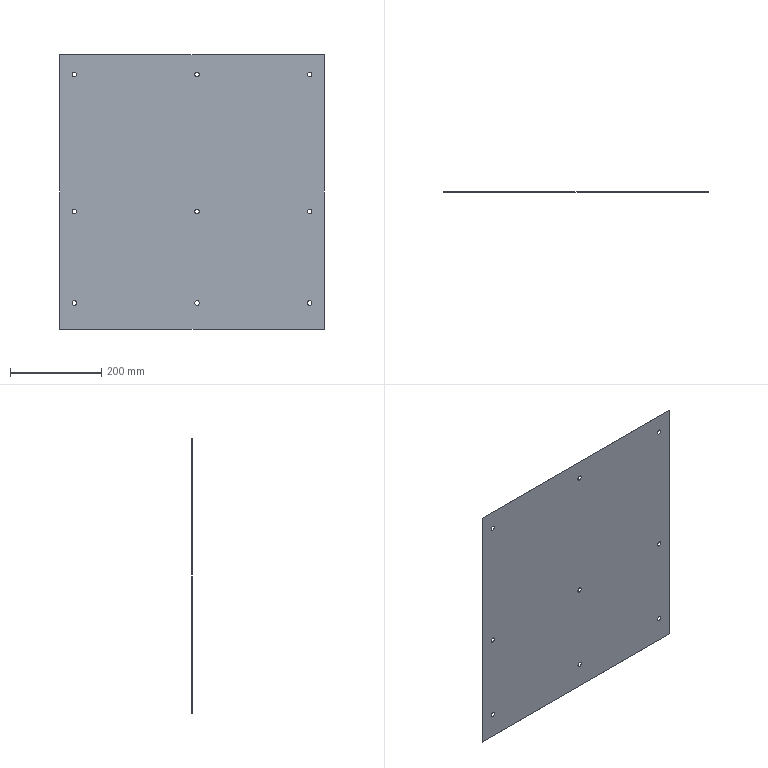Part | SolidWorks | features LPattern 2, Extrusion 1, FlatPattern 1, HoleWzd 1, SheetMetal 1, SolidToSheetMetal 1 | 1 solid | 24 faces | box 580 x 0.18 x 600 mm | volume 62513 mm3 | cylinder 18 | plane 6 | commonest cylinder face diameters 10 x18
STEP:
#1=CARTESIAN_POINT('',(301.2,0.18,52.));
#2=VERTEX_POINT('',#1);
#3=CARTESIAN_POINT('',(301.2,0.18,62.));
#4=VERTEX_POINT('',#3);
#5=CARTESIAN_POINT('',(301.2,0.18,57.));
#6=DIRECTION('',(0.,1.,0.));
#7=DIRECTION('',(0.,0.,1.));
#8=AXIS2_PLACEMENT_3D('',#5,#6,#7);
#9=CIRCLE('',#8,5.);
#10=EDGE_CURVE('',#2,#4,#9,.T.);
#11=ORIENTED_EDGE('',*,*,#10,.T.);
#12=CARTESIAN_POINT('',(301.2,0.,62.));
#13=VERTEX_POINT('',#12);
#14=CARTESIAN_POINT('',(301.2,0.,62.));
#15=DIRECTION('',(0.,-1.,0.));
#16=VECTOR('',#15,1000.);
#17=LINE('',#14,#16);
#18=EDGE_CURVE('',#4,#13,#17,.T.);
#19=ORIENTED_EDGE('',*,*,#18,.T.);
#20=CARTESIAN_POINT('',(301.2,0.,52.));
#21=VERTEX_POINT('',#20);
#22=CARTESIAN_POINT('',(301.2,0.,57.));
#23=DIRECTION('',(0.,-1.,0.));
#24=DIRECTION('',(0.,0.,-1.));
#25=AXIS2_PLACEMENT_3D('',#22,#23,#24);
#26=CIRCLE('',#25,5.);
#27=EDGE_CURVE('',#13,#21,#26,.T.);
#28=ORIENTED_EDGE('',*,*,#27,.T.);
#29=CARTESIAN_POINT('',(301.2,0.,52.));
#30=DIRECTION('',(0.,-1.,0.));
#31=VECTOR('',#30,1000.);
#32=LINE('',#29,#31);
#33=EDGE_CURVE('',#2,#21,#32,.T.);
#34=ORIENTED_EDGE('',*,*,#33,.F.);
#35=EDGE_LOOP('',(#11,#19,#28,#34));
#36=FACE_OUTER_BOUND('',#35,.T.);
#37=CARTESIAN_POINT('',(301.2,0.,57.));
#38=DIRECTION('',(0.,-1.,0.));
#39=DIRECTION('',(0.,0.,-1.));
#40=AXIS2_PLACEMENT_3D('',#37,#38,#39);
#41=CYLINDRICAL_SURFACE('',#40,5.);
#42=ADVANCED_FACE('',(#36),#41,.F.);
#43=CARTESIAN_POINT('',(32.4,0.18,52.));
#44=VERTEX_POINT('',#43);
#45=CARTESIAN_POINT('',(32.4,0.18,62.));
#46=VERTEX_POINT('',#45);
#47=CARTESIAN_POINT('',(32.4,0.18,57.));
#48=DIRECTION('',(0.,1.,0.));
#49=DIRECTION('',(0.,0.,1.));
#50=AXIS2_PLACEMENT_3D('',#47,#48,#49);
#51=CIRCLE('',#50,5.);
#52=EDGE_CURVE('',#44,#46,#51,.T.);
#53=ORIENTED_EDGE('',*,*,#52,.T.);
#54=CARTESIAN_POINT('',(32.4,0.,62.));
#55=VERTEX_POINT('',#54);
#56=CARTESIAN_POINT('',(32.4,0.,62.));
#57=DIRECTION('',(0.,-1.,0.));
#58=VECTOR('',#57,1000.);
#59=LINE('',#56,#58);
#60=EDGE_CURVE('',#46,#55,#59,.T.);
#61=ORIENTED_EDGE('',*,*,#60,.T.);
#62=CARTESIAN_POINT('',(32.4,0.,52.));
#63=VERTEX_POINT('',#62);
#64=CARTESIAN_POINT('',(32.4,0.,57.));
#65=DIRECTION('',(0.,-1.,0.));
#66=DIRECTION('',(0.,0.,-1.));
#67=AXIS2_PLACEMENT_3D('',#64,#65,#66);
#68=CIRCLE('',#67,5.);
#69=EDGE_CURVE('',#55,#63,#68,.T.);
#70=ORIENTED_EDGE('',*,*,#69,.T.);
#71=CARTESIAN_POINT('',(32.4,0.,52.));
#72=DIRECTION('',(0.,-1.,0.));
#73=VECTOR('',#72,1000.);
#74=LINE('',#71,#73);
#75=EDGE_CURVE('',#44,#63,#74,.T.);
#76=ORIENTED_EDGE('',*,*,#75,.F.);
#77=EDGE_LOOP('',(#53,#61,#70,#76));
#78=FACE_OUTER_BOUND('',#77,.T.);
#79=CARTESIAN_POINT('',(32.4,0.,57.));
#80=DIRECTION('',(0.,-1.,0.));
#81=DIRECTION('',(0.,0.,-1.));
#82=AXIS2_PLACEMENT_3D('',#79,#80,#81);
#83=CYLINDRICAL_SURFACE('',#82,5.);
#84=ADVANCED_FACE('',(#78),#83,.F.);
#85=CARTESIAN_POINT('',(547.6,0.18,52.));
#86=VERTEX_POINT('',#85);
#87=CARTESIAN_POINT('',(547.6,0.18,62.));
#88=VERTEX_POINT('',#87);
#89=CARTESIAN_POINT('',(547.6,0.18,57.));
#90=DIRECTION('',(0.,1.,0.));
#91=DIRECTION('',(0.,0.,1.));
#92=AXIS2_PLACEMENT_3D('',#89,#90,#91);
#93=CIRCLE('',#92,5.);
#94=EDGE_CURVE('',#86,#88,#93,.T.);
#95=ORIENTED_EDGE('',*,*,#94,.T.);
#96=CARTESIAN_POINT('',(547.6,0.,62.));
#97=VERTEX_POINT('',#96);
#98=CARTESIAN_POINT('',(547.6,0.,62.));
#99=DIRECTION('',(0.,-1.,0.));
#100=VECTOR('',#99,1000.);
#101=LINE('',#98,#100);
#102=EDGE_CURVE('',#88,#97,#101,.T.);
#103=ORIENTED_EDGE('',*,*,#102,.T.);
#104=CARTESIAN_POINT('',(547.6,0.,52.));
#105=VERTEX_POINT('',#104);
#106=CARTESIAN_POINT('',(547.6,0.,57.));
#107=DIRECTION('',(0.,-1.,0.));
#108=DIRECTION('',(0.,0.,-1.));
#109=AXIS2_PLACEMENT_3D('',#106,#107,#108);
#110=CIRCLE('',#109,5.);
#111=EDGE_CURVE('',#97,#105,#110,.T.);
#112=ORIENTED_EDGE('',*,*,#111,.T.);
#113=CARTESIAN_POINT('',(547.6,0.,52.));
#114=DIRECTION('',(0.,-1.,0.));
#115=VECTOR('',#114,1000.);
#116=LINE('',#113,#115);
#117=EDGE_CURVE('',#86,#105,#116,.T.);
#118=ORIENTED_EDGE('',*,*,#117,.F.);
#119=EDGE_LOOP('',(#95,#103,#112,#118));
#120=FACE_OUTER_BOUND('',#119,.T.);
#121=CARTESIAN_POINT('',(547.6,0.,57.));
#122=DIRECTION('',(0.,-1.,0.));
#123=DIRECTION('',(0.,0.,-1.));
#124=AXIS2_PLACEMENT_3D('',#121,#122,#123);
#125=CYLINDRICAL_SURFACE('',#124,5.);
#126=ADVANCED_FACE('',(#120),#125,.F.);
#127=CARTESIAN_POINT('',(301.2,0.18,252.));
#128=VERTEX_POINT('',#127);
#129=CARTESIAN_POINT('',(301.2,0.18,262.));
#130=VERTEX_POINT('',#129);
#131=CARTESIAN_POINT('',(301.2,0.18,257.));
#132=DIRECTION('',(0.,1.,0.));
#133=DIRECTION('',(0.,0.,1.));
#134=AXIS2_PLACEMENT_3D('',#131,#132,#133);
#135=CIRCLE('',#134,5.);
#136=EDGE_CURVE('',#128,#130,#135,.T.);
#137=ORIENTED_EDGE('',*,*,#136,.T.);
#138=CARTESIAN_POINT('',(301.2,0.,262.));
#139=VERTEX_POINT('',#138);
#140=CARTESIAN_POINT('',(301.2,0.,262.));
#141=DIRECTION('',(0.,-1.,0.));
#142=VECTOR('',#141,1000.);
#143=LINE('',#140,#142);
#144=EDGE_CURVE('',#130,#139,#143,.T.);
#145=ORIENTED_EDGE('',*,*,#144,.T.);
#146=CARTESIAN_POINT('',(301.2,0.,252.));
#147=VERTEX_POINT('',#146);
#148=CARTESIAN_POINT('',(301.2,0.,257.));
#149=DIRECTION('',(0.,-1.,0.));
#150=DIRECTION('',(0.,0.,-1.));
#151=AXIS2_PLACEMENT_3D('',#148,#149,#150);
#152=CIRCLE('',#151,5.);
#153=EDGE_CURVE('',#139,#147,#152,.T.);
#154=ORIENTED_EDGE('',*,*,#153,.T.);
#155=CARTESIAN_POINT('',(301.2,0.,252.));
#156=DIRECTION('',(0.,-1.,0.));
#157=VECTOR('',#156,1000.);
#158=LINE('',#155,#157);
#159=EDGE_CURVE('',#128,#147,#158,.T.);
#160=ORIENTED_EDGE('',*,*,#159,.F.);
#161=EDGE_LOOP('',(#137,#145,#154,#160));
#162=FACE_OUTER_BOUND('',#161,.T.);
#163=CARTESIAN_POINT('',(301.2,0.,257.));
#164=DIRECTION('',(0.,-1.,0.));
#165=DIRECTION('',(0.,0.,-1.));
#166=AXIS2_PLACEMENT_3D('',#163,#164,#165);
#167=CYLINDRICAL_SURFACE('',#166,5.);
#168=ADVANCED_FACE('',(#162),#167,.F.);
#169=CARTESIAN_POINT('',(32.4,0.18,252.));
#170=VERTEX_POINT('',#169);
#171=CARTESIAN_POINT('',(32.4,0.18,262.));
#172=VERTEX_POINT('',#171);
#173=CARTESIAN_POINT('',(32.4,0.18,257.));
#174=DIRECTION('',(0.,1.,0.));
#175=DIRECTION('',(0.,0.,1.));
#176=AXIS2_PLACEMENT_3D('',#173,#174,#175);
#177=CIRCLE('',#176,5.);
#178=EDGE_CURVE('',#170,#172,#177,.T.);
#179=ORIENTED_EDGE('',*,*,#178,.T.);
#180=CARTESIAN_POINT('',(32.4,0.,262.));
#181=VERTEX_POINT('',#180);
#182=CARTESIAN_POINT('',(32.4,0.,262.));
#183=DIRECTION('',(0.,-1.,0.));
#184=VECTOR('',#183,1000.);
#185=LINE('',#182,#184);
#186=EDGE_CURVE('',#172,#181,#185,.T.);
#187=ORIENTED_EDGE('',*,*,#186,.T.);
#188=CARTESIAN_POINT('',(32.4,0.,252.));
#189=VERTEX_POINT('',#188);
#190=CARTESIAN_POINT('',(32.4,0.,257.));
#191=DIRECTION('',(0.,-1.,0.));
#192=DIRECTION('',(0.,0.,-1.));
#193=AXIS2_PLACEMENT_3D('',#190,#191,#192);
#194=CIRCLE('',#193,5.);
#195=EDGE_CURVE('',#181,#189,#194,.T.);
#196=ORIENTED_EDGE('',*,*,#195,.T.);
#197=CARTESIAN_POINT('',(32.4,0.,252.));
#198=DIRECTION('',(0.,-1.,0.));
#199=VECTOR('',#198,1000.);
#200=LINE('',#197,#199);
#201=EDGE_CURVE('',#170,#189,#200,.T.);
#202=ORIENTED_EDGE('',*,*,#201,.F.);
#203=EDGE_LOOP('',(#179,#187,#196,#202));
#204=FACE_OUTER_BOUND('',#203,.T.);
#205=CARTESIAN_POINT('',(32.4,0.,257.));
#206=DIRECTION('',(0.,-1.,0.));
#207=DIRECTION('',(0.,0.,-1.));
#208=AXIS2_PLACEMENT_3D('',#205,#206,#207);
#209=CYLINDRICAL_SURFACE('',#208,5.);
#210=ADVANCED_FACE('',(#204),#209,.F.);
#211=CARTESIAN_POINT('',(547.6,0.18,252.));
#212=VERTEX_POINT('',#211);
#213=CARTESIAN_POINT('',(547.6,0.18,262.));
#214=VERTEX_POINT('',#213);
#215=CARTESIAN_POINT('',(547.6,0.18,257.));
#216=DIRECTION('',(0.,1.,0.));
#217=DIRECTION('',(0.,0.,1.));
#218=AXIS2_PLACEMENT_3D('',#215,#216,#217);
#219=CIRCLE('',#218,5.);
#220=EDGE_CURVE('',#212,#214,#219,.T.);
#221=ORIENTED_EDGE('',*,*,#220,.T.);
#222=CARTESIAN_POINT('',(547.6,0.,262.));
#223=VERTEX_POINT('',#222);
#224=CARTESIAN_POINT('',(547.6,0.,262.));
#225=DIRECTION('',(0.,-1.,0.));
#226=VECTOR('',#225,1000.);
#227=LINE('',#224,#226);
#228=EDGE_CURVE('',#214,#223,#227,.T.);
#229=ORIENTED_EDGE('',*,*,#228,.T.);
#230=CARTESIAN_POINT('',(547.6,0.,252.));
#231=VERTEX_POINT('',#230);
#232=CARTESIAN_POINT('',(547.6,0.,257.));
#233=DIRECTION('',(0.,-1.,0.));
#234=DIRECTION('',(0.,0.,-1.));
#235=AXIS2_PLACEMENT_3D('',#232,#233,#234);
#236=CIRCLE('',#235,5.);
#237=EDGE_CURVE('',#223,#231,#236,.T.);
#238=ORIENTED_EDGE('',*,*,#237,.T.);
#239=CARTESIAN_POINT('',(547.6,0.,252.));
#240=DIRECTION('',(0.,-1.,0.));
#241=VECTOR('',#240,1000.);
#242=LINE('',#239,#241);
#243=EDGE_CURVE('',#212,#231,#242,.T.);
#244=ORIENTED_EDGE('',*,*,#243,.F.);
#245=EDGE_LOOP('',(#221,#229,#238,#244));
#246=FACE_OUTER_BOUND('',#245,.T.);
#247=CARTESIAN_POINT('',(547.6,0.,257.));
#248=DIRECTION('',(0.,-1.,0.));
#249=DIRECTION('',(0.,0.,-1.));
#250=AXIS2_PLACEMENT_3D('',#247,#248,#249);
#251=CYLINDRICAL_SURFACE('',#250,5.);
#252=ADVANCED_FACE('',(#246),#251,.F.);
#253=CARTESIAN_POINT('',(547.6,0.18,552.));
#254=VERTEX_POINT('',#253);
#255=CARTESIAN_POINT('',(547.6,0.18,562.));
#256=VERTEX_POINT('',#255);
#257=CARTESIAN_POINT('',(547.6,0.18,557.));
#258=DIRECTION('',(0.,1.,0.));
#259=DIRECTION('',(0.,0.,1.));
#260=AXIS2_PLACEMENT_3D('',#257,#258,#259);
#261=CIRCLE('',#260,5.);
#262=EDGE_CURVE('',#254,#256,#261,.T.);
#263=ORIENTED_EDGE('',*,*,#262,.T.);
#264=CARTESIAN_POINT('',(547.6,0.,562.));
#265=VERTEX_POINT('',#264);
#266=CARTESIAN_POINT('',(547.6,0.,562.));
#267=DIRECTION('',(0.,-1.,0.));
#268=VECTOR('',#267,1000.);
#269=LINE('',#266,#268);
#270=EDGE_CURVE('',#256,#265,#269,.T.);
#271=ORIENTED_EDGE('',*,*,#270,.T.);
#272=CARTESIAN_POINT('',(547.6,0.,552.));
#273=VERTEX_POINT('',#272);
#274=CARTESIAN_POINT('',(547.6,0.,557.));
#275=DIRECTION('',(0.,-1.,0.));
#276=DIRECTION('',(0.,0.,-1.));
#277=AXIS2_PLACEMENT_3D('',#274,#275,#276);
#278=CIRCLE('',#277,5.);
#279=EDGE_CURVE('',#265,#273,#278,.T.);
#280=ORIENTED_EDGE('',*,*,#279,.T.);
#281=CARTESIAN_POINT('',(547.6,0.,552.));
#282=DIRECTION('',(0.,-1.,0.));
#283=VECTOR('',#282,1000.);
#284=LINE('',#281,#283);
#285=EDGE_CURVE('',#254,#273,#284,.T.);
#286=ORIENTED_EDGE('',*,*,#285,.F.);
#287=EDGE_LOOP('',(#263,#271,#280,#286));
#288=FACE_OUTER_BOUND('',#287,.T.);
#289=CARTESIAN_POINT('',(547.6,0.,557.));
#290=DIRECTION('',(0.,-1.,0.));
#291=DIRECTION('',(0.,0.,-1.));
#292=AXIS2_PLACEMENT_3D('',#289,#290,#291);
#293=CYLINDRICAL_SURFACE('',#292,5.);
#294=ADVANCED_FACE('',(#288),#293,.F.);
#295=CARTESIAN_POINT('',(301.2,0.18,552.));
#296=VERTEX_POINT('',#295);
#297=CARTESIAN_POINT('',(301.2,0.18,562.));
#298=VERTEX_POINT('',#297);
#299=CARTESIAN_POINT('',(301.2,0.18,557.));
#300=DIRECTION('',(0.,1.,0.));
#301=DIRECTION('',(0.,0.,1.));
#302=AXIS2_PLACEMENT_3D('',#299,#300,#301);
#303=CIRCLE('',#302,5.);
#304=EDGE_CURVE('',#296,#298,#303,.T.);
#305=ORIENTED_EDGE('',*,*,#304,.T.);
#306=CARTESIAN_POINT('',(301.2,0.,562.));
#307=VERTEX_POINT('',#306);
#308=CARTESIAN_POINT('',(301.2,0.,562.));
#309=DIRECTION('',(0.,-1.,0.));
#310=VECTOR('',#309,1000.);
#311=LINE('',#308,#310);
#312=EDGE_CURVE('',#298,#307,#311,.T.);
#313=ORIENTED_EDGE('',*,*,#312,.T.);
#314=CARTESIAN_POINT('',(301.2,0.,552.));
#315=VERTEX_POINT('',#314);
#316=CARTESIAN_POINT('',(301.2,0.,557.));
#317=DIRECTION('',(0.,-1.,0.));
#318=DIRECTION('',(0.,0.,-1.));
#319=AXIS2_PLACEMENT_3D('',#316,#317,#318);
#320=CIRCLE('',#319,5.);
#321=EDGE_CURVE('',#307,#315,#320,.T.);
#322=ORIENTED_EDGE('',*,*,#321,.T.);
#323=CARTESIAN_POINT('',(301.2,0.,552.));
#324=DIRECTION('',(0.,-1.,0.));
#325=VECTOR('',#324,1000.);
#326=LINE('',#323,#325);
#327=EDGE_CURVE('',#296,#315,#326,.T.);
#328=ORIENTED_EDGE('',*,*,#327,.F.);
#329=EDGE_LOOP('',(#305,#313,#322,#328));
#330=FACE_OUTER_BOUND('',#329,.T.);
#331=CARTESIAN_POINT('',(301.2,0.,557.));
#332=DIRECTION('',(0.,-1.,0.));
#333=DIRECTION('',(0.,0.,-1.));
#334=AXIS2_PLACEMENT_3D('',#331,#332,#333);
#335=CYLINDRICAL_SURFACE('',#334,5.);
#336=ADVANCED_FACE('',(#330),#335,.F.);
#337=CARTESIAN_POINT('',(32.4,0.18,552.));
#338=VERTEX_POINT('',#337);
#339=CARTESIAN_POINT('',(32.4,0.18,562.));
#340=VERTEX_POINT('',#339);
#341=CARTESIAN_POINT('',(32.4,0.18,557.));
#342=DIRECTION('',(0.,1.,0.));
#343=DIRECTION('',(0.,0.,1.));
#344=AXIS2_PLACEMENT_3D('',#341,#342,#343);
#345=CIRCLE('',#344,5.);
#346=EDGE_CURVE('',#338,#340,#345,.T.);
#347=ORIENTED_EDGE('',*,*,#346,.T.);
#348=CARTESIAN_POINT('',(32.4,0.,562.));
#349=VERTEX_POINT('',#348);
#350=CARTESIAN_POINT('',(32.4,0.,562.));
#351=DIRECTION('',(0.,-1.,0.));
#352=VECTOR('',#351,1000.);
#353=LINE('',#350,#352);
#354=EDGE_CURVE('',#340,#349,#353,.T.);
#355=ORIENTED_EDGE('',*,*,#354,.T.);
#356=CARTESIAN_POINT('',(32.4,0.,552.));
#357=VERTEX_POINT('',#356);
#358=CARTESIAN_POINT('',(32.4,0.,557.));
#359=DIRECTION('',(0.,-1.,0.));
#360=DIRECTION('',(0.,0.,-1.));
#361=AXIS2_PLACEMENT_3D('',#358,#359,#360);
#362=CIRCLE('',#361,5.);
#363=EDGE_CURVE('',#349,#357,#362,.T.);
#364=ORIENTED_EDGE('',*,*,#363,.T.);
#365=CARTESIAN_POINT('',(32.4,0.,552.));
#366=DIRECTION('',(0.,-1.,0.));
#367=VECTOR('',#366,1000.);
#368=LINE('',#365,#367);
#369=EDGE_CURVE('',#338,#357,#368,.T.);
#370=ORIENTED_EDGE('',*,*,#369,.F.);
#371=EDGE_LOOP('',(#347,#355,#364,#370));
#372=FACE_OUTER_BOUND('',#371,.T.);
#373=CARTESIAN_POINT('',(32.4,0.,557.));
#374=DIRECTION('',(0.,-1.,0.));
#375=DIRECTION('',(0.,0.,-1.));
#376=AXIS2_PLACEMENT_3D('',#373,#374,#375);
#377=CYLINDRICAL_SURFACE('',#376,5.);
#378=ADVANCED_FACE('',(#372),#377,.F.);
#379=CARTESIAN_POINT('',(580.,0.,600.));
#380=VERTEX_POINT('',#379);
#381=CARTESIAN_POINT('',(580.,0.18,600.));
#382=VERTEX_POINT('',#381);
#383=CARTESIAN_POINT('',(580.,0.18,600.));
#384=DIRECTION('',(0.,1.,0.));
#385=VECTOR('',#384,1000.);
#386=LINE('',#383,#385);
#387=EDGE_CURVE('',#380,#382,#386,.T.);
#388=ORIENTED_EDGE('',*,*,#387,.F.);
#389=CARTESIAN_POINT('',(580.,0.,0.));
#390=VERTEX_POINT('',#389);
#391=CARTESIAN_POINT('',(580.,0.,0.));
#392=DIRECTION('',(0.,0.,-1.));
#393=VECTOR('',#392,1000.);
#394=LINE('',#391,#393);
#395=EDGE_CURVE('',#380,#390,#394,.T.);
#396=ORIENTED_EDGE('',*,*,#395,.T.);
#397=CARTESIAN_POINT('',(580.,0.18,0.));
#398=VERTEX_POINT('',#397);
#399=CARTESIAN_POINT('',(580.,0.18,0.));
#400=DIRECTION('',(0.,1.,0.));
#401=VECTOR('',#400,1000.);
#402=LINE('',#399,#401);
#403=EDGE_CURVE('',#390,#398,#402,.T.);
#404=ORIENTED_EDGE('',*,*,#403,.T.);
#405=CARTESIAN_POINT('',(580.,0.18,0.));
#406=DIRECTION('',(0.,0.,-1.));
#407=VECTOR('',#406,1000.);
#408=LINE('',#405,#407);
#409=EDGE_CURVE('',#382,#398,#408,.T.);
#410=ORIENTED_EDGE('',*,*,#409,.F.);
#411=EDGE_LOOP('',(#388,#396,#404,#410));
#412=FACE_OUTER_BOUND('',#411,.T.);
#413=CARTESIAN_POINT('',(580.,0.18,0.));
#414=DIRECTION('',(1.,0.,0.));
#415=DIRECTION('',(0.,0.,-1.));
#416=AXIS2_PLACEMENT_3D('',#413,#414,#415);
#417=PLANE('',#416);
#418=ADVANCED_FACE('',(#412),#417,.T.);
#419=ORIENTED_EDGE('',*,*,#403,.F.);
#420=CARTESIAN_POINT('',(0.,0.,0.));
#421=VERTEX_POINT('',#420);
#422=CARTESIAN_POINT('',(0.,0.,0.));
#423=DIRECTION('',(-1.,0.,0.));
#424=VECTOR('',#423,1000.);
#425=LINE('',#422,#424);
#426=EDGE_CURVE('',#390,#421,#425,.T.);
#427=ORIENTED_EDGE('',*,*,#426,.T.);
#428=CARTESIAN_POINT('',(0.,0.18,0.));
#429=VERTEX_POINT('',#428);
#430=CARTESIAN_POINT('',(0.,0.18,0.));
#431=DIRECTION('',(0.,1.,0.));
#432=VECTOR('',#431,1000.);
#433=LINE('',#430,#432);
#434=EDGE_CURVE('',#421,#429,#433,.T.);
#435=ORIENTED_EDGE('',*,*,#434,.T.);
#436=CARTESIAN_POINT('',(0.,0.18,0.));
#437=DIRECTION('',(-1.,0.,0.));
#438=VECTOR('',#437,1000.);
#439=LINE('',#436,#438);
#440=EDGE_CURVE('',#398,#429,#439,.T.);
#441=ORIENTED_EDGE('',*,*,#440,.F.);
#442=EDGE_LOOP('',(#419,#427,#435,#441));
#443=FACE_OUTER_BOUND('',#442,.T.);
#444=CARTESIAN_POINT('',(0.,0.18,0.));
#445=DIRECTION('',(0.,0.,-1.));
#446=DIRECTION('',(-1.,0.,0.));
#447=AXIS2_PLACEMENT_3D('',#444,#445,#446);
#448=PLANE('',#447);
#449=ADVANCED_FACE('',(#443),#448,.T.);
#450=ORIENTED_EDGE('',*,*,#434,.F.);
#451=CARTESIAN_POINT('',(0.,0.,600.));
#452=VERTEX_POINT('',#451);
#453=CARTESIAN_POINT('',(0.,0.,0.));
#454=DIRECTION('',(0.,0.,1.));
#455=VECTOR('',#454,1000.);
#456=LINE('',#453,#455);
#457=EDGE_CURVE('',#421,#452,#456,.T.);
#458=ORIENTED_EDGE('',*,*,#457,.T.);
#459=CARTESIAN_POINT('',(0.,0.18,600.));
#460=VERTEX_POINT('',#459);
#461=CARTESIAN_POINT('',(0.,0.18,600.));
#462=DIRECTION('',(0.,1.,0.));
#463=VECTOR('',#462,1000.);
#464=LINE('',#461,#463);
#465=EDGE_CURVE('',#452,#460,#464,.T.);
#466=ORIENTED_EDGE('',*,*,#465,.T.);
#467=CARTESIAN_POINT('',(0.,0.18,0.));
#468=DIRECTION('',(0.,0.,1.));
#469=VECTOR('',#468,1000.);
#470=LINE('',#467,#469);
#471=EDGE_CURVE('',#429,#460,#470,.T.);
#472=ORIENTED_EDGE('',*,*,#471,.F.);
#473=EDGE_LOOP('',(#450,#458,#466,#472));
#474=FACE_OUTER_BOUND('',#473,.T.);
#475=CARTESIAN_POINT('',(0.,0.18,0.));
#476=DIRECTION('',(-1.,0.,0.));
#477=DIRECTION('',(0.,0.,1.));
#478=AXIS2_PLACEMENT_3D('',#475,#476,#477);
#479=PLANE('',#478);
#480=ADVANCED_FACE('',(#474),#479,.T.);
#481=CARTESIAN_POINT('',(0.,0.,600.));
#482=DIRECTION('',(1.,0.,0.));
#483=VECTOR('',#482,1000.);
#484=LINE('',#481,#483);
#485=EDGE_CURVE('',#452,#380,#484,.T.);
#486=ORIENTED_EDGE('',*,*,#485,.T.);
#487=ORIENTED_EDGE('',*,*,#387,.T.);
#488=CARTESIAN_POINT('',(0.,0.18,600.));
#489=DIRECTION('',(1.,0.,0.));
#490=VECTOR('',#489,1000.);
#491=LINE('',#488,#490);
#492=EDGE_CURVE('',#460,#382,#491,.T.);
#493=ORIENTED_EDGE('',*,*,#492,.F.);
#494=ORIENTED_EDGE('',*,*,#465,.F.);
#495=EDGE_LOOP('',(#486,#487,#493,#494));
#496=FACE_OUTER_BOUND('',#495,.T.);
#497=CARTESIAN_POINT('',(0.,0.18,600.));
#498=DIRECTION('',(0.,0.,1.));
#499=DIRECTION('',(1.,0.,0.));
#500=AXIS2_PLACEMENT_3D('',#497,#498,#499);
#501=PLANE('',#500);
#502=ADVANCED_FACE('',(#496),#501,.T.);
#503=ORIENTED_EDGE('',*,*,#10,.F.);
#504=CARTESIAN_POINT('',(301.2,0.18,57.));
#505=DIRECTION('',(0.,1.,0.));
#506=DIRECTION('',(0.,0.,1.));
#507=AXIS2_PLACEMENT_3D('',#504,#505,#506);
#508=CIRCLE('',#507,5.);
#509=EDGE_CURVE('',#4,#2,#508,.T.);
#510=ORIENTED_EDGE('',*,*,#509,.F.);
#511=EDGE_LOOP('',(#503,#510));
#512=FACE_BOUND('',#511,.T.);
#513=ORIENTED_EDGE('',*,*,#52,.F.);
#514=CARTESIAN_POINT('',(32.4,0.18,57.));
#515=DIRECTION('',(0.,1.,0.));
#516=DIRECTION('',(0.,0.,1.));
#517=AXIS2_PLACEMENT_3D('',#514,#515,#516);
#518=CIRCLE('',#517,5.);
#519=EDGE_CURVE('',#46,#44,#518,.T.);
#520=ORIENTED_EDGE('',*,*,#519,.F.);
#521=EDGE_LOOP('',(#513,#520));
#522=FACE_BOUND('',#521,.T.);
#523=ORIENTED_EDGE('',*,*,#94,.F.);
#524=CARTESIAN_POINT('',(547.6,0.18,57.));
#525=DIRECTION('',(0.,1.,0.));
#526=DIRECTION('',(0.,0.,1.));
#527=AXIS2_PLACEMENT_3D('',#524,#525,#526);
#528=CIRCLE('',#527,5.);
#529=EDGE_CURVE('',#88,#86,#528,.T.);
#530=ORIENTED_EDGE('',*,*,#529,.F.);
#531=EDGE_LOOP('',(#523,#530));
#532=FACE_BOUND('',#531,.T.);
#533=ORIENTED_EDGE('',*,*,#136,.F.);
#534=CARTESIAN_POINT('',(301.2,0.18,257.));
#535=DIRECTION('',(0.,1.,0.));
#536=DIRECTION('',(0.,0.,1.));
#537=AXIS2_PLACEMENT_3D('',#534,#535,#536);
#538=CIRCLE('',#537,5.);
#539=EDGE_CURVE('',#130,#128,#538,.T.);
#540=ORIENTED_EDGE('',*,*,#539,.F.);
#541=EDGE_LOOP('',(#533,#540));
#542=FACE_BOUND('',#541,.T.);
#543=ORIENTED_EDGE('',*,*,#178,.F.);
#544=CARTESIAN_POINT('',(32.4,0.18,257.));
#545=DIRECTION('',(0.,1.,0.));
#546=DIRECTION('',(0.,0.,1.));
#547=AXIS2_PLACEMENT_3D('',#544,#545,#546);
#548=CIRCLE('',#547,5.);
#549=EDGE_CURVE('',#172,#170,#548,.T.);
#550=ORIENTED_EDGE('',*,*,#549,.F.);
#551=EDGE_LOOP('',(#543,#550));
#552=FACE_BOUND('',#551,.T.);
#553=ORIENTED_EDGE('',*,*,#220,.F.);
#554=CARTESIAN_POINT('',(547.6,0.18,257.));
#555=DIRECTION('',(0.,1.,0.));
#556=DIRECTION('',(0.,0.,1.));
#557=AXIS2_PLACEMENT_3D('',#554,#555,#556);
#558=CIRCLE('',#557,5.);
#559=EDGE_CURVE('',#214,#212,#558,.T.);
#560=ORIENTED_EDGE('',*,*,#559,.F.);
#561=EDGE_LOOP('',(#553,#560));
#562=FACE_BOUND('',#561,.T.);
#563=ORIENTED_EDGE('',*,*,#262,.F.);
#564=CARTESIAN_POINT('',(547.6,0.18,557.));
#565=DIRECTION('',(0.,1.,0.));
#566=DIRECTION('',(0.,0.,1.));
#567=AXIS2_PLACEMENT_3D('',#564,#565,#566);
#568=CIRCLE('',#567,5.);
#569=EDGE_CURVE('',#256,#254,#568,.T.);
#570=ORIENTED_EDGE('',*,*,#569,.F.);
#571=EDGE_LOOP('',(#563,#570));
#572=FACE_BOUND('',#571,.T.);
#573=ORIENTED_EDGE('',*,*,#304,.F.);
#574=CARTESIAN_POINT('',(301.2,0.18,557.));
#575=DIRECTION('',(0.,1.,0.));
#576=DIRECTION('',(0.,0.,1.));
#577=AXIS2_PLACEMENT_3D('',#574,#575,#576);
#578=CIRCLE('',#577,5.);
#579=EDGE_CURVE('',#298,#296,#578,.T.);
#580=ORIENTED_EDGE('',*,*,#579,.F.);
#581=EDGE_LOOP('',(#573,#580));
#582=FACE_BOUND('',#581,.T.);
#583=ORIENTED_EDGE('',*,*,#346,.F.);
#584=CARTESIAN_POINT('',(32.4,0.18,557.));
#585=DIRECTION('',(0.,1.,0.));
#586=DIRECTION('',(0.,0.,1.));
#587=AXIS2_PLACEMENT_3D('',#584,#585,#586);
#588=CIRCLE('',#587,5.);
#589=EDGE_CURVE('',#340,#338,#588,.T.);
#590=ORIENTED_EDGE('',*,*,#589,.F.);
#591=EDGE_LOOP('',(#583,#590));
#592=FACE_BOUND('',#591,.T.);
#593=ORIENTED_EDGE('',*,*,#471,.T.);
#594=ORIENTED_EDGE('',*,*,#492,.T.);
#595=ORIENTED_EDGE('',*,*,#409,.T.);
#596=ORIENTED_EDGE('',*,*,#440,.T.);
#597=EDGE_LOOP('',(#593,#594,#595,#596));
#598=FACE_OUTER_BOUND('',#597,.T.);
#599=CARTESIAN_POINT('',(0.,0.18,0.));
#600=DIRECTION('',(0.,1.,0.));
#601=DIRECTION('',(0.,0.,1.));
#602=AXIS2_PLACEMENT_3D('',#599,#600,#601);
#603=PLANE('',#602);
#604=ADVANCED_FACE('',(#512,#522,#532,#542,#552,#562,#572,#582,#592,#598),#603,.T.);
#605=CARTESIAN_POINT('',(301.2,0.,57.));
#606=DIRECTION('',(0.,-1.,0.));
#607=DIRECTION('',(0.,0.,-1.));
#608=AXIS2_PLACEMENT_3D('',#605,#606,#607);
#609=CIRCLE('',#608,5.);
#610=EDGE_CURVE('',#21,#13,#609,.T.);
#611=ORIENTED_EDGE('',*,*,#610,.F.);
#612=ORIENTED_EDGE('',*,*,#27,.F.);
#613=EDGE_LOOP('',(#611,#612));
#614=FACE_BOUND('',#613,.T.);
#615=CARTESIAN_POINT('',(32.4,0.,57.));
#616=DIRECTION('',(0.,-1.,0.));
#617=DIRECTION('',(0.,0.,-1.));
#618=AXIS2_PLACEMENT_3D('',#615,#616,#617);
#619=CIRCLE('',#618,5.);
#620=EDGE_CURVE('',#63,#55,#619,.T.);
#621=ORIENTED_EDGE('',*,*,#620,.F.);
#622=ORIENTED_EDGE('',*,*,#69,.F.);
#623=EDGE_LOOP('',(#621,#622));
#624=FACE_BOUND('',#623,.T.);
#625=CARTESIAN_POINT('',(547.6,0.,57.));
#626=DIRECTION('',(0.,-1.,0.));
#627=DIRECTION('',(0.,0.,-1.));
#628=AXIS2_PLACEMENT_3D('',#625,#626,#627);
#629=CIRCLE('',#628,5.);
#630=EDGE_CURVE('',#105,#97,#629,.T.);
#631=ORIENTED_EDGE('',*,*,#630,.F.);
#632=ORIENTED_EDGE('',*,*,#111,.F.);
#633=EDGE_LOOP('',(#631,#632));
#634=FACE_BOUND('',#633,.T.);
#635=CARTESIAN_POINT('',(301.2,0.,257.));
#636=DIRECTION('',(0.,-1.,0.));
#637=DIRECTION('',(0.,0.,-1.));
#638=AXIS2_PLACEMENT_3D('',#635,#636,#637);
#639=CIRCLE('',#638,5.);
#640=EDGE_CURVE('',#147,#139,#639,.T.);
#641=ORIENTED_EDGE('',*,*,#640,.F.);
#642=ORIENTED_EDGE('',*,*,#153,.F.);
#643=EDGE_LOOP('',(#641,#642));
#644=FACE_BOUND('',#643,.T.);
#645=CARTESIAN_POINT('',(32.4,0.,257.));
#646=DIRECTION('',(0.,-1.,0.));
#647=DIRECTION('',(0.,0.,-1.));
#648=AXIS2_PLACEMENT_3D('',#645,#646,#647);
#649=CIRCLE('',#648,5.);
#650=EDGE_CURVE('',#189,#181,#649,.T.);
#651=ORIENTED_EDGE('',*,*,#650,.F.);
#652=ORIENTED_EDGE('',*,*,#195,.F.);
#653=EDGE_LOOP('',(#651,#652));
#654=FACE_BOUND('',#653,.T.);
#655=CARTESIAN_POINT('',(547.6,0.,257.));
#656=DIRECTION('',(0.,-1.,0.));
#657=DIRECTION('',(0.,0.,-1.));
#658=AXIS2_PLACEMENT_3D('',#655,#656,#657);
#659=CIRCLE('',#658,5.);
#660=EDGE_CURVE('',#231,#223,#659,.T.);
#661=ORIENTED_EDGE('',*,*,#660,.F.);
#662=ORIENTED_EDGE('',*,*,#237,.F.);
#663=EDGE_LOOP('',(#661,#662));
#664=FACE_BOUND('',#663,.T.);
#665=CARTESIAN_POINT('',(547.6,0.,557.));
#666=DIRECTION('',(0.,-1.,0.));
#667=DIRECTION('',(0.,0.,-1.));
#668=AXIS2_PLACEMENT_3D('',#665,#666,#667);
#669=CIRCLE('',#668,5.);
#670=EDGE_CURVE('',#273,#265,#669,.T.);
#671=ORIENTED_EDGE('',*,*,#670,.F.);
#672=ORIENTED_EDGE('',*,*,#279,.F.);
#673=EDGE_LOOP('',(#671,#672));
#674=FACE_BOUND('',#673,.T.);
#675=CARTESIAN_POINT('',(301.2,0.,557.));
#676=DIRECTION('',(0.,-1.,0.));
#677=DIRECTION('',(0.,0.,-1.));
#678=AXIS2_PLACEMENT_3D('',#675,#676,#677);
#679=CIRCLE('',#678,5.);
#680=EDGE_CURVE('',#315,#307,#679,.T.);
#681=ORIENTED_EDGE('',*,*,#680,.F.);
#682=ORIENTED_EDGE('',*,*,#321,.F.);
#683=EDGE_LOOP('',(#681,#682));
#684=FACE_BOUND('',#683,.T.);
#685=CARTESIAN_POINT('',(32.4,0.,557.));
#686=DIRECTION('',(0.,-1.,0.));
#687=DIRECTION('',(0.,0.,-1.));
#688=AXIS2_PLACEMENT_3D('',#685,#686,#687);
#689=CIRCLE('',#688,5.);
#690=EDGE_CURVE('',#357,#349,#689,.T.);
#691=ORIENTED_EDGE('',*,*,#690,.F.);
#692=ORIENTED_EDGE('',*,*,#363,.F.);
#693=EDGE_LOOP('',(#691,#692));
#694=FACE_BOUND('',#693,.T.);
#695=ORIENTED_EDGE('',*,*,#457,.F.);
#696=ORIENTED_EDGE('',*,*,#426,.F.);
#697=ORIENTED_EDGE('',*,*,#395,.F.);
#698=ORIENTED_EDGE('',*,*,#485,.F.);
#699=EDGE_LOOP('',(#695,#696,#697,#698));
#700=FACE_OUTER_BOUND('',#699,.T.);
#701=CARTESIAN_POINT('',(0.,0.,0.));
#702=DIRECTION('',(0.,1.,0.));
#703=DIRECTION('',(0.,0.,1.));
#704=AXIS2_PLACEMENT_3D('',#701,#702,#703);
#705=PLANE('',#704);
#706=ADVANCED_FACE('',(#614,#624,#634,#644,#654,#664,#674,#684,#694,#700),#705,.F.);
#707=ORIENTED_EDGE('',*,*,#354,.F.);
#708=ORIENTED_EDGE('',*,*,#589,.T.);
#709=ORIENTED_EDGE('',*,*,#369,.T.);
#710=ORIENTED_EDGE('',*,*,#690,.T.);
#711=EDGE_LOOP('',(#707,#708,#709,#710));
#712=FACE_OUTER_BOUND('',#711,.T.);
#713=CARTESIAN_POINT('',(32.4,0.,557.));
#714=DIRECTION('',(0.,-1.,0.));
#715=DIRECTION('',(0.,0.,-1.));
#716=AXIS2_PLACEMENT_3D('',#713,#714,#715);
#717=CYLINDRICAL_SURFACE('',#716,5.);
#718=ADVANCED_FACE('',(#712),#717,.F.);
#719=ORIENTED_EDGE('',*,*,#312,.F.);
#720=ORIENTED_EDGE('',*,*,#579,.T.);
#721=ORIENTED_EDGE('',*,*,#327,.T.);
#722=ORIENTED_EDGE('',*,*,#680,.T.);
#723=EDGE_LOOP('',(#719,#720,#721,#722));
#724=FACE_OUTER_BOUND('',#723,.T.);
#725=CARTESIAN_POINT('',(301.2,0.,557.));
#726=DIRECTION('',(0.,-1.,0.));
#727=DIRECTION('',(0.,0.,-1.));
#728=AXIS2_PLACEMENT_3D('',#725,#726,#727);
#729=CYLINDRICAL_SURFACE('',#728,5.);
#730=ADVANCED_FACE('',(#724),#729,.F.);
#731=ORIENTED_EDGE('',*,*,#270,.F.);
#732=ORIENTED_EDGE('',*,*,#569,.T.);
#733=ORIENTED_EDGE('',*,*,#285,.T.);
#734=ORIENTED_EDGE('',*,*,#670,.T.);
#735=EDGE_LOOP('',(#731,#732,#733,#734));
#736=FACE_OUTER_BOUND('',#735,.T.);
#737=CARTESIAN_POINT('',(547.6,0.,557.));
#738=DIRECTION('',(0.,-1.,0.));
#739=DIRECTION('',(0.,0.,-1.));
#740=AXIS2_PLACEMENT_3D('',#737,#738,#739);
#741=CYLINDRICAL_SURFACE('',#740,5.);
#742=ADVANCED_FACE('',(#736),#741,.F.);
#743=ORIENTED_EDGE('',*,*,#228,.F.);
#744=ORIENTED_EDGE('',*,*,#559,.T.);
#745=ORIENTED_EDGE('',*,*,#243,.T.);
#746=ORIENTED_EDGE('',*,*,#660,.T.);
#747=EDGE_LOOP('',(#743,#744,#745,#746));
#748=FACE_OUTER_BOUND('',#747,.T.);
#749=CARTESIAN_POINT('',(547.6,0.,257.));
#750=DIRECTION('',(0.,-1.,0.));
#751=DIRECTION('',(0.,0.,-1.));
#752=AXIS2_PLACEMENT_3D('',#749,#750,#751);
#753=CYLINDRICAL_SURFACE('',#752,5.);
#754=ADVANCED_FACE('',(#748),#753,.F.);
#755=ORIENTED_EDGE('',*,*,#186,.F.);
#756=ORIENTED_EDGE('',*,*,#549,.T.);
#757=ORIENTED_EDGE('',*,*,#201,.T.);
#758=ORIENTED_EDGE('',*,*,#650,.T.);
#759=EDGE_LOOP('',(#755,#756,#757,#758));
#760=FACE_OUTER_BOUND('',#759,.T.);
#761=CARTESIAN_POINT('',(32.4,0.,257.));
#762=DIRECTION('',(0.,-1.,0.));
#763=DIRECTION('',(0.,0.,-1.));
#764=AXIS2_PLACEMENT_3D('',#761,#762,#763);
#765=CYLINDRICAL_SURFACE('',#764,5.);
#766=ADVANCED_FACE('',(#760),#765,.F.);
#767=ORIENTED_EDGE('',*,*,#144,.F.);
#768=ORIENTED_EDGE('',*,*,#539,.T.);
#769=ORIENTED_EDGE('',*,*,#159,.T.);
#770=ORIENTED_EDGE('',*,*,#640,.T.);
#771=EDGE_LOOP('',(#767,#768,#769,#770));
#772=FACE_OUTER_BOUND('',#771,.T.);
#773=CARTESIAN_POINT('',(301.2,0.,257.));
#774=DIRECTION('',(0.,-1.,0.));
#775=DIRECTION('',(0.,0.,-1.));
#776=AXIS2_PLACEMENT_3D('',#773,#774,#775);
#777=CYLINDRICAL_SURFACE('',#776,5.);
#778=ADVANCED_FACE('',(#772),#777,.F.);
#779=ORIENTED_EDGE('',*,*,#102,.F.);
#780=ORIENTED_EDGE('',*,*,#529,.T.);
#781=ORIENTED_EDGE('',*,*,#117,.T.);
#782=ORIENTED_EDGE('',*,*,#630,.T.);
#783=EDGE_LOOP('',(#779,#780,#781,#782));
#784=FACE_OUTER_BOUND('',#783,.T.);
#785=CARTESIAN_POINT('',(547.6,0.,57.));
#786=DIRECTION('',(0.,-1.,0.));
#787=DIRECTION('',(0.,0.,-1.));
#788=AXIS2_PLACEMENT_3D('',#785,#786,#787);
#789=CYLINDRICAL_SURFACE('',#788,5.);
#790=ADVANCED_FACE('',(#784),#789,.F.);
#791=ORIENTED_EDGE('',*,*,#60,.F.);
#792=ORIENTED_EDGE('',*,*,#519,.T.);
#793=ORIENTED_EDGE('',*,*,#75,.T.);
#794=ORIENTED_EDGE('',*,*,#620,.T.);
#795=EDGE_LOOP('',(#791,#792,#793,#794));
#796=FACE_OUTER_BOUND('',#795,.T.);
#797=CARTESIAN_POINT('',(32.4,0.,57.));
#798=DIRECTION('',(0.,-1.,0.));
#799=DIRECTION('',(0.,0.,-1.));
#800=AXIS2_PLACEMENT_3D('',#797,#798,#799);
#801=CYLINDRICAL_SURFACE('',#800,5.);
#802=ADVANCED_FACE('',(#796),#801,.F.);
#803=ORIENTED_EDGE('',*,*,#18,.F.);
#804=ORIENTED_EDGE('',*,*,#509,.T.);
#805=ORIENTED_EDGE('',*,*,#33,.T.);
#806=ORIENTED_EDGE('',*,*,#610,.T.);
#807=EDGE_LOOP('',(#803,#804,#805,#806));
#808=FACE_OUTER_BOUND('',#807,.T.);
#809=CARTESIAN_POINT('',(301.2,0.,57.));
#810=DIRECTION('',(0.,-1.,0.));
#811=DIRECTION('',(0.,0.,-1.));
#812=AXIS2_PLACEMENT_3D('',#809,#810,#811);
#813=CYLINDRICAL_SURFACE('',#812,5.);
#814=ADVANCED_FACE('',(#808),#813,.F.);
#815=CLOSED_SHELL('',(#42,#84,#126,#168,#210,#252,#294,#336,#378,#418,#449,#480,#502,#604,#706,#718,#730,#742,#754,#766,#778,#790,#802,#814));
#816=MANIFOLD_SOLID_BREP('',#815);
#817=CARTESIAN_POINT('',(0.,0.,0.));
#818=DIRECTION('',(0.,0.,1.));
#819=DIRECTION('',(1.,0.,0.));
#820=AXIS2_PLACEMENT_3D('',#817,#818,#819);
#821=(LENGTH_UNIT()NAMED_UNIT(*)SI_UNIT(.MILLI.,.METRE.));
#822=UNCERTAINTY_MEASURE_WITH_UNIT(LENGTH_MEASURE(0.00001),#821,'','');
#823=(NAMED_UNIT(*)PLANE_ANGLE_UNIT()SI_UNIT($,.RADIAN.));
#824=(NAMED_UNIT(*)SI_UNIT($,.STERADIAN.)SOLID_ANGLE_UNIT());
#825=(GEOMETRIC_REPRESENTATION_CONTEXT(3)GLOBAL_UNCERTAINTY_ASSIGNED_CONTEXT((#822))GLOBAL_UNIT_ASSIGNED_CONTEXT((#821,#823,#824))REPRESENTATION_CONTEXT('',''));
#826=ADVANCED_BREP_SHAPE_REPRESENTATION('',(#816,#820),#825);